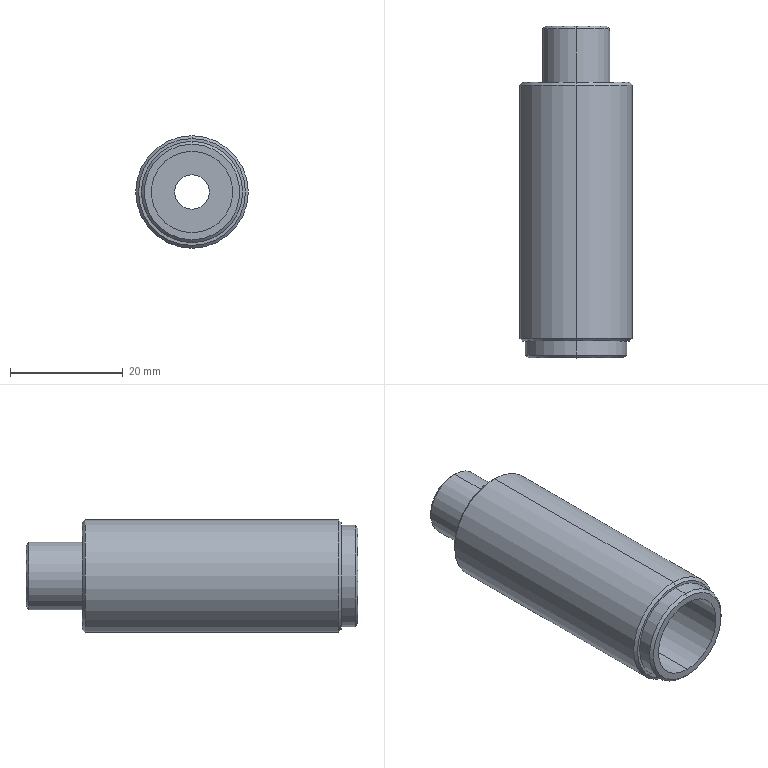Part | STEP file | 1 solid | 23 faces | box 20 x 59 x 20 mm | volume 11876 mm3 | cylinder 10 | cone 8 | plane 5 | commonest cylinder face diameters 6.1 x2 12 x2 14.5 x2 18 x2 20 x2
STEP:
#1=CARTESIAN_POINT('',(0.,0.,0.));
#2=DIRECTION('',(0.,0.,1.));
#3=DIRECTION('',(1.,0.,0.));
#4=AXIS2_PLACEMENT_3D('',#1,#2,#3);
#5=CARTESIAN_POINT('',(0.,10.,5.5));
#6=VERTEX_POINT('',#5);
#7=CARTESIAN_POINT('',(0.,10.,-5.5));
#8=VERTEX_POINT('',#7);
#9=CARTESIAN_POINT('',(0.,10.,0.));
#10=DIRECTION('',(0.,1.,0.));
#11=DIRECTION('',(0.,0.,1.));
#12=AXIS2_PLACEMENT_3D('',#9,#10,#11);
#13=CIRCLE('',#12,5.5);
#14=CARTESIAN_POINT('',(0.,10.,0.));
#15=DIRECTION('',(0.,-1.,0.));
#16=DIRECTION('',(0.,0.,-1.));
#17=AXIS2_PLACEMENT_3D('',#14,#15,#16);
#18=CONICAL_SURFACE('',#17,5.5,0.7854);
#19=CARTESIAN_POINT('',(3.142,0.));
#20=DIRECTION('',(-1.,0.));
#21=VECTOR('',#20,1.);
#22=LINE('',#19,#21);
#23=(GEOMETRIC_REPRESENTATION_CONTEXT(2)PARAMETRIC_REPRESENTATION_CONTEXT()REPRESENTATION_CONTEXT('',''));
#24=DEFINITIONAL_REPRESENTATION('',(#22),#23);
#25=PCURVE('',#18,#24);
#26=CARTESIAN_POINT('',(0.,10.,0.));
#27=DIRECTION('',(0.,1.,0.));
#28=DIRECTION('',(0.,0.,1.));
#29=AXIS2_PLACEMENT_3D('',#26,#27,#28);
#30=PLANE('',#29);
#31=CARTESIAN_POINT('',(0.,0.));
#32=DIRECTION('',(1.,0.));
#33=AXIS2_PLACEMENT_2D('',#31,#32);
#34=CIRCLE('',#33,5.5);
#35=(GEOMETRIC_REPRESENTATION_CONTEXT(2)PARAMETRIC_REPRESENTATION_CONTEXT()REPRESENTATION_CONTEXT('',''));
#36=DEFINITIONAL_REPRESENTATION('',(#34),#35);
#37=PCURVE('',#30,#36);
#38=SURFACE_CURVE('',#13,(#25,#37),.PCURVE_S1.);
#39=EDGE_CURVE('',#6,#8,#38,.T.);
#40=ORIENTED_EDGE('',*,*,#39,.F.);
#41=CARTESIAN_POINT('',(0.,9.5,6.));
#42=VERTEX_POINT('',#41);
#43=CARTESIAN_POINT('',(0.,10.,5.5));
#44=DIRECTION('',(0.,-0.7071,0.7071));
#45=VECTOR('',#44,1.);
#46=LINE('',#43,#45);
#47=CARTESIAN_POINT('',(3.142,0.));
#48=DIRECTION('',(0.,1.));
#49=VECTOR('',#48,1.);
#50=LINE('',#47,#49);
#51=(GEOMETRIC_REPRESENTATION_CONTEXT(2)PARAMETRIC_REPRESENTATION_CONTEXT()REPRESENTATION_CONTEXT('',''));
#52=DEFINITIONAL_REPRESENTATION('',(#50),#51);
#53=PCURVE('',#18,#52);
#54=CARTESIAN_POINT('',(0.,10.,0.));
#55=DIRECTION('',(0.,-1.,0.));
#56=DIRECTION('',(0.,0.,-1.));
#57=AXIS2_PLACEMENT_3D('',#54,#55,#56);
#58=CONICAL_SURFACE('',#57,5.5,0.7854);
#59=CARTESIAN_POINT('',(3.142,0.));
#60=DIRECTION('',(0.,1.));
#61=VECTOR('',#60,1.);
#62=LINE('',#59,#61);
#63=(GEOMETRIC_REPRESENTATION_CONTEXT(2)PARAMETRIC_REPRESENTATION_CONTEXT()REPRESENTATION_CONTEXT('',''));
#64=DEFINITIONAL_REPRESENTATION('',(#62),#63);
#65=PCURVE('',#58,#64);
#66=SURFACE_CURVE('',#46,(#53,#65),.PCURVE_S1.);
#67=EDGE_CURVE('',#6,#42,#66,.T.);
#68=ORIENTED_EDGE('',*,*,#67,.T.);
#69=CARTESIAN_POINT('',(0.,9.5,-6.));
#70=VERTEX_POINT('',#69);
#71=CARTESIAN_POINT('',(0.,9.5,0.));
#72=DIRECTION('',(0.,-1.,0.));
#73=DIRECTION('',(0.,0.,1.));
#74=AXIS2_PLACEMENT_3D('',#71,#72,#73);
#75=CIRCLE('',#74,6.);
#76=CARTESIAN_POINT('',(-3.142,0.5));
#77=DIRECTION('',(1.,0.));
#78=VECTOR('',#77,1.);
#79=LINE('',#76,#78);
#80=(GEOMETRIC_REPRESENTATION_CONTEXT(2)PARAMETRIC_REPRESENTATION_CONTEXT()REPRESENTATION_CONTEXT('',''));
#81=DEFINITIONAL_REPRESENTATION('',(#79),#80);
#82=PCURVE('',#18,#81);
#83=CARTESIAN_POINT('',(0.,10.,0.));
#84=DIRECTION('',(0.,-1.,0.));
#85=DIRECTION('',(0.,0.,-1.));
#86=AXIS2_PLACEMENT_3D('',#83,#84,#85);
#87=CYLINDRICAL_SURFACE('',#86,6.);
#88=CARTESIAN_POINT('',(-3.142,0.5));
#89=DIRECTION('',(1.,0.));
#90=VECTOR('',#89,1.);
#91=LINE('',#88,#90);
#92=(GEOMETRIC_REPRESENTATION_CONTEXT(2)PARAMETRIC_REPRESENTATION_CONTEXT()REPRESENTATION_CONTEXT('',''));
#93=DEFINITIONAL_REPRESENTATION('',(#91),#92);
#94=PCURVE('',#87,#93);
#95=SURFACE_CURVE('',#75,(#82,#94),.PCURVE_S1.);
#96=EDGE_CURVE('',#70,#42,#95,.T.);
#97=ORIENTED_EDGE('',*,*,#96,.F.);
#98=CARTESIAN_POINT('',(0.,10.,-5.5));
#99=DIRECTION('',(0.,-0.7071,-0.7071));
#100=VECTOR('',#99,1.);
#101=LINE('',#98,#100);
#102=CARTESIAN_POINT('',(0.,0.));
#103=DIRECTION('',(0.,1.));
#104=VECTOR('',#103,1.);
#105=LINE('',#102,#104);
#106=(GEOMETRIC_REPRESENTATION_CONTEXT(2)PARAMETRIC_REPRESENTATION_CONTEXT()REPRESENTATION_CONTEXT('',''));
#107=DEFINITIONAL_REPRESENTATION('',(#105),#106);
#108=PCURVE('',#18,#107);
#109=CARTESIAN_POINT('',(6.283,0.));
#110=DIRECTION('',(0.,1.));
#111=VECTOR('',#110,1.);
#112=LINE('',#109,#111);
#113=(GEOMETRIC_REPRESENTATION_CONTEXT(2)PARAMETRIC_REPRESENTATION_CONTEXT()REPRESENTATION_CONTEXT('',''));
#114=DEFINITIONAL_REPRESENTATION('',(#112),#113);
#115=PCURVE('',#58,#114);
#116=SURFACE_CURVE('',#101,(#108,#115),.PCURVE_S1.);
#117=EDGE_CURVE('',#8,#70,#116,.T.);
#118=ORIENTED_EDGE('',*,*,#117,.F.);
#119=EDGE_LOOP('',(#40,#68,#97,#118));
#120=FACE_BOUND('',#119,.T.);
#121=ADVANCED_FACE('',(#120),#18,.T.);
#122=CARTESIAN_POINT('',(0.,-49.,-8.5));
#123=VERTEX_POINT('',#122);
#124=CARTESIAN_POINT('',(0.,-49.,8.5));
#125=VERTEX_POINT('',#124);
#126=CARTESIAN_POINT('',(0.,-49.,0.));
#127=DIRECTION('',(0.,-1.,0.));
#128=DIRECTION('',(0.,0.,1.));
#129=AXIS2_PLACEMENT_3D('',#126,#127,#128);
#130=CIRCLE('',#129,8.5);
#131=CARTESIAN_POINT('',(0.,-49.,0.));
#132=DIRECTION('',(0.,1.,0.));
#133=DIRECTION('',(0.,0.,1.));
#134=AXIS2_PLACEMENT_3D('',#131,#132,#133);
#135=CONICAL_SURFACE('',#134,8.5,0.7854);
#136=CARTESIAN_POINT('',(6.283,0.));
#137=DIRECTION('',(-1.,0.));
#138=VECTOR('',#137,1.);
#139=LINE('',#136,#138);
#140=(GEOMETRIC_REPRESENTATION_CONTEXT(2)PARAMETRIC_REPRESENTATION_CONTEXT()REPRESENTATION_CONTEXT('',''));
#141=DEFINITIONAL_REPRESENTATION('',(#139),#140);
#142=PCURVE('',#135,#141);
#143=CARTESIAN_POINT('',(0.,-49.,0.));
#144=DIRECTION('',(0.,1.,0.));
#145=DIRECTION('',(0.,0.,1.));
#146=AXIS2_PLACEMENT_3D('',#143,#144,#145);
#147=PLANE('',#146);
#148=CARTESIAN_POINT('',(8.5,0.));
#149=CARTESIAN_POINT('',(8.5,-14.722));
#150=CARTESIAN_POINT('',(-4.25,-7.361));
#151=CARTESIAN_POINT('',(-17.,0.));
#152=CARTESIAN_POINT('',(-4.25,7.361));
#153=CARTESIAN_POINT('',(8.5,14.722));
#154=CARTESIAN_POINT('',(8.5,0.));
#155=(BOUNDED_CURVE()B_SPLINE_CURVE(2,(#148,#149,#150,#151,#152,#153,#154),.UNSPECIFIED.,.T.,.F.)B_SPLINE_CURVE_WITH_KNOTS((1,2,2,2,2,1),(-2.094,0.,2.094,4.189,6.283,8.378),.UNSPECIFIED.)CURVE()GEOMETRIC_REPRESENTATION_ITEM()RATIONAL_B_SPLINE_CURVE((1.,0.5,1.,0.5,1.,0.5,1.))REPRESENTATION_ITEM(''));
#156=(GEOMETRIC_REPRESENTATION_CONTEXT(2)PARAMETRIC_REPRESENTATION_CONTEXT()REPRESENTATION_CONTEXT('',''));
#157=DEFINITIONAL_REPRESENTATION('',(#155),#156);
#158=PCURVE('',#147,#157);
#159=SURFACE_CURVE('',#130,(#142,#158),.PCURVE_S1.);
#160=EDGE_CURVE('',#123,#125,#159,.T.);
#161=ORIENTED_EDGE('',*,*,#160,.F.);
#162=CARTESIAN_POINT('',(0.,-48.5,-9.));
#163=VERTEX_POINT('',#162);
#164=CARTESIAN_POINT('',(0.,-49.,-8.5));
#165=DIRECTION('',(0.,0.7071,-0.7071));
#166=VECTOR('',#165,1.);
#167=LINE('',#164,#166);
#168=CARTESIAN_POINT('',(3.142,0.));
#169=DIRECTION('',(0.,1.));
#170=VECTOR('',#169,1.);
#171=LINE('',#168,#170);
#172=(GEOMETRIC_REPRESENTATION_CONTEXT(2)PARAMETRIC_REPRESENTATION_CONTEXT()REPRESENTATION_CONTEXT('',''));
#173=DEFINITIONAL_REPRESENTATION('',(#171),#172);
#174=PCURVE('',#135,#173);
#175=CARTESIAN_POINT('',(0.,-49.,0.));
#176=DIRECTION('',(0.,1.,0.));
#177=DIRECTION('',(0.,0.,1.));
#178=AXIS2_PLACEMENT_3D('',#175,#176,#177);
#179=CONICAL_SURFACE('',#178,8.5,0.7854);
#180=CARTESIAN_POINT('',(3.142,0.));
#181=DIRECTION('',(0.,1.));
#182=VECTOR('',#181,1.);
#183=LINE('',#180,#182);
#184=(GEOMETRIC_REPRESENTATION_CONTEXT(2)PARAMETRIC_REPRESENTATION_CONTEXT()REPRESENTATION_CONTEXT('',''));
#185=DEFINITIONAL_REPRESENTATION('',(#183),#184);
#186=PCURVE('',#179,#185);
#187=SURFACE_CURVE('',#167,(#174,#186),.PCURVE_S1.);
#188=EDGE_CURVE('',#123,#163,#187,.T.);
#189=ORIENTED_EDGE('',*,*,#188,.T.);
#190=CARTESIAN_POINT('',(0.,-48.5,9.));
#191=VERTEX_POINT('',#190);
#192=CARTESIAN_POINT('',(0.,-48.5,0.));
#193=DIRECTION('',(0.,1.,0.));
#194=DIRECTION('',(0.,0.,1.));
#195=AXIS2_PLACEMENT_3D('',#192,#193,#194);
#196=CIRCLE('',#195,9.);
#197=CARTESIAN_POINT('',(0.,0.5));
#198=DIRECTION('',(1.,0.));
#199=VECTOR('',#198,1.);
#200=LINE('',#197,#199);
#201=(GEOMETRIC_REPRESENTATION_CONTEXT(2)PARAMETRIC_REPRESENTATION_CONTEXT()REPRESENTATION_CONTEXT('',''));
#202=DEFINITIONAL_REPRESENTATION('',(#200),#201);
#203=PCURVE('',#135,#202);
#204=CARTESIAN_POINT('',(0.,-46.,0.));
#205=DIRECTION('',(0.,-1.,0.));
#206=DIRECTION('',(0.,0.,-1.));
#207=AXIS2_PLACEMENT_3D('',#204,#205,#206);
#208=CYLINDRICAL_SURFACE('',#207,9.);
#209=CARTESIAN_POINT('',(3.142,2.5));
#210=DIRECTION('',(-1.,0.));
#211=VECTOR('',#210,1.);
#212=LINE('',#209,#211);
#213=(GEOMETRIC_REPRESENTATION_CONTEXT(2)PARAMETRIC_REPRESENTATION_CONTEXT()REPRESENTATION_CONTEXT('',''));
#214=DEFINITIONAL_REPRESENTATION('',(#212),#213);
#215=PCURVE('',#208,#214);
#216=SURFACE_CURVE('',#196,(#203,#215),.PCURVE_S1.);
#217=EDGE_CURVE('',#191,#163,#216,.T.);
#218=ORIENTED_EDGE('',*,*,#217,.F.);
#219=CARTESIAN_POINT('',(0.,-49.,8.5));
#220=DIRECTION('',(0.,0.7071,0.7071));
#221=VECTOR('',#220,1.);
#222=LINE('',#219,#221);
#223=CARTESIAN_POINT('',(0.,0.));
#224=DIRECTION('',(0.,1.));
#225=VECTOR('',#224,1.);
#226=LINE('',#223,#225);
#227=(GEOMETRIC_REPRESENTATION_CONTEXT(2)PARAMETRIC_REPRESENTATION_CONTEXT()REPRESENTATION_CONTEXT('',''));
#228=DEFINITIONAL_REPRESENTATION('',(#226),#227);
#229=PCURVE('',#135,#228);
#230=CARTESIAN_POINT('',(6.283,0.));
#231=DIRECTION('',(0.,1.));
#232=VECTOR('',#231,1.);
#233=LINE('',#230,#232);
#234=(GEOMETRIC_REPRESENTATION_CONTEXT(2)PARAMETRIC_REPRESENTATION_CONTEXT()REPRESENTATION_CONTEXT('',''));
#235=DEFINITIONAL_REPRESENTATION('',(#233),#234);
#236=PCURVE('',#179,#235);
#237=SURFACE_CURVE('',#222,(#229,#236),.PCURVE_S1.);
#238=EDGE_CURVE('',#125,#191,#237,.T.);
#239=ORIENTED_EDGE('',*,*,#238,.F.);
#240=EDGE_LOOP('',(#161,#189,#218,#239));
#241=FACE_BOUND('',#240,.T.);
#242=ADVANCED_FACE('',(#241),#135,.T.);
#243=CARTESIAN_POINT('',(0.,0.,9.5));
#244=VERTEX_POINT('',#243);
#245=CARTESIAN_POINT('',(0.,0.,-9.5));
#246=VERTEX_POINT('',#245);
#247=CARTESIAN_POINT('',(0.,0.,0.));
#248=DIRECTION('',(0.,1.,0.));
#249=DIRECTION('',(0.,0.,1.));
#250=AXIS2_PLACEMENT_3D('',#247,#248,#249);
#251=CIRCLE('',#250,9.5);
#252=CARTESIAN_POINT('',(0.,0.,0.));
#253=DIRECTION('',(0.,-1.,0.));
#254=DIRECTION('',(0.,0.,-1.));
#255=AXIS2_PLACEMENT_3D('',#252,#253,#254);
#256=CONICAL_SURFACE('',#255,9.5,0.7854);
#257=CARTESIAN_POINT('',(3.142,0.));
#258=DIRECTION('',(-1.,0.));
#259=VECTOR('',#258,1.);
#260=LINE('',#257,#259);
#261=(GEOMETRIC_REPRESENTATION_CONTEXT(2)PARAMETRIC_REPRESENTATION_CONTEXT()REPRESENTATION_CONTEXT('',''));
#262=DEFINITIONAL_REPRESENTATION('',(#260),#261);
#263=PCURVE('',#256,#262);
#264=CARTESIAN_POINT('',(0.,0.,0.));
#265=DIRECTION('',(0.,1.,0.));
#266=DIRECTION('',(0.,0.,1.));
#267=AXIS2_PLACEMENT_3D('',#264,#265,#266);
#268=PLANE('',#267);
#269=CARTESIAN_POINT('',(0.,0.));
#270=DIRECTION('',(1.,0.));
#271=AXIS2_PLACEMENT_2D('',#269,#270);
#272=CIRCLE('',#271,9.5);
#273=(GEOMETRIC_REPRESENTATION_CONTEXT(2)PARAMETRIC_REPRESENTATION_CONTEXT()REPRESENTATION_CONTEXT('',''));
#274=DEFINITIONAL_REPRESENTATION('',(#272),#273);
#275=PCURVE('',#268,#274);
#276=SURFACE_CURVE('',#251,(#263,#275),.PCURVE_S1.);
#277=EDGE_CURVE('',#244,#246,#276,.T.);
#278=ORIENTED_EDGE('',*,*,#277,.F.);
#279=CARTESIAN_POINT('',(0.,-0.5,10.));
#280=VERTEX_POINT('',#279);
#281=CARTESIAN_POINT('',(0.,0.,9.5));
#282=DIRECTION('',(0.,-0.7071,0.7071));
#283=VECTOR('',#282,1.);
#284=LINE('',#281,#283);
#285=CARTESIAN_POINT('',(3.142,0.));
#286=DIRECTION('',(0.,1.));
#287=VECTOR('',#286,1.);
#288=LINE('',#285,#287);
#289=(GEOMETRIC_REPRESENTATION_CONTEXT(2)PARAMETRIC_REPRESENTATION_CONTEXT()REPRESENTATION_CONTEXT('',''));
#290=DEFINITIONAL_REPRESENTATION('',(#288),#289);
#291=PCURVE('',#256,#290);
#292=CARTESIAN_POINT('',(0.,0.,0.));
#293=DIRECTION('',(0.,-1.,0.));
#294=DIRECTION('',(0.,0.,-1.));
#295=AXIS2_PLACEMENT_3D('',#292,#293,#294);
#296=CONICAL_SURFACE('',#295,9.5,0.7854);
#297=CARTESIAN_POINT('',(3.142,0.));
#298=DIRECTION('',(0.,1.));
#299=VECTOR('',#298,1.);
#300=LINE('',#297,#299);
#301=(GEOMETRIC_REPRESENTATION_CONTEXT(2)PARAMETRIC_REPRESENTATION_CONTEXT()REPRESENTATION_CONTEXT('',''));
#302=DEFINITIONAL_REPRESENTATION('',(#300),#301);
#303=PCURVE('',#296,#302);
#304=SURFACE_CURVE('',#284,(#291,#303),.PCURVE_S1.);
#305=EDGE_CURVE('',#244,#280,#304,.T.);
#306=ORIENTED_EDGE('',*,*,#305,.T.);
#307=CARTESIAN_POINT('',(0.,-0.5,-10.));
#308=VERTEX_POINT('',#307);
#309=CARTESIAN_POINT('',(0.,-0.5,0.));
#310=DIRECTION('',(0.,-1.,0.));
#311=DIRECTION('',(0.,0.,1.));
#312=AXIS2_PLACEMENT_3D('',#309,#310,#311);
#313=CIRCLE('',#312,10.);
#314=CARTESIAN_POINT('',(-3.142,0.5));
#315=DIRECTION('',(1.,0.));
#316=VECTOR('',#315,1.);
#317=LINE('',#314,#316);
#318=(GEOMETRIC_REPRESENTATION_CONTEXT(2)PARAMETRIC_REPRESENTATION_CONTEXT()REPRESENTATION_CONTEXT('',''));
#319=DEFINITIONAL_REPRESENTATION('',(#317),#318);
#320=PCURVE('',#256,#319);
#321=CARTESIAN_POINT('',(0.,-49.,0.));
#322=DIRECTION('',(0.,1.,0.));
#323=DIRECTION('',(0.,0.,1.));
#324=AXIS2_PLACEMENT_3D('',#321,#322,#323);
#325=CYLINDRICAL_SURFACE('',#324,10.);
#326=CARTESIAN_POINT('',(6.283,48.5));
#327=DIRECTION('',(-1.,0.));
#328=VECTOR('',#327,1.);
#329=LINE('',#326,#328);
#330=(GEOMETRIC_REPRESENTATION_CONTEXT(2)PARAMETRIC_REPRESENTATION_CONTEXT()REPRESENTATION_CONTEXT('',''));
#331=DEFINITIONAL_REPRESENTATION('',(#329),#330);
#332=PCURVE('',#325,#331);
#333=SURFACE_CURVE('',#313,(#320,#332),.PCURVE_S1.);
#334=EDGE_CURVE('',#308,#280,#333,.T.);
#335=ORIENTED_EDGE('',*,*,#334,.F.);
#336=CARTESIAN_POINT('',(0.,0.,-9.5));
#337=DIRECTION('',(0.,-0.7071,-0.7071));
#338=VECTOR('',#337,1.);
#339=LINE('',#336,#338);
#340=CARTESIAN_POINT('',(0.,0.));
#341=DIRECTION('',(0.,1.));
#342=VECTOR('',#341,1.);
#343=LINE('',#340,#342);
#344=(GEOMETRIC_REPRESENTATION_CONTEXT(2)PARAMETRIC_REPRESENTATION_CONTEXT()REPRESENTATION_CONTEXT('',''));
#345=DEFINITIONAL_REPRESENTATION('',(#343),#344);
#346=PCURVE('',#256,#345);
#347=CARTESIAN_POINT('',(6.283,0.));
#348=DIRECTION('',(0.,1.));
#349=VECTOR('',#348,1.);
#350=LINE('',#347,#349);
#351=(GEOMETRIC_REPRESENTATION_CONTEXT(2)PARAMETRIC_REPRESENTATION_CONTEXT()REPRESENTATION_CONTEXT('',''));
#352=DEFINITIONAL_REPRESENTATION('',(#350),#351);
#353=PCURVE('',#296,#352);
#354=SURFACE_CURVE('',#339,(#346,#353),.PCURVE_S1.);
#355=EDGE_CURVE('',#246,#308,#354,.T.);
#356=ORIENTED_EDGE('',*,*,#355,.F.);
#357=EDGE_LOOP('',(#278,#306,#335,#356));
#358=FACE_BOUND('',#357,.T.);
#359=ADVANCED_FACE('',(#358),#256,.T.);
#360=CARTESIAN_POINT('',(0.,-46.,-9.5));
#361=VERTEX_POINT('',#360);
#362=CARTESIAN_POINT('',(0.,-46.,9.5));
#363=VERTEX_POINT('',#362);
#364=CARTESIAN_POINT('',(0.,-46.,0.));
#365=DIRECTION('',(0.,-1.,0.));
#366=DIRECTION('',(0.,0.,-1.));
#367=AXIS2_PLACEMENT_3D('',#364,#365,#366);
#368=CIRCLE('',#367,9.5);
#369=CARTESIAN_POINT('',(0.,-46.,0.));
#370=DIRECTION('',(0.,1.,0.));
#371=DIRECTION('',(0.,0.,1.));
#372=AXIS2_PLACEMENT_3D('',#369,#370,#371);
#373=CONICAL_SURFACE('',#372,9.5,0.7854);
#374=CARTESIAN_POINT('',(3.142,0.));
#375=DIRECTION('',(-1.,0.));
#376=VECTOR('',#375,1.);
#377=LINE('',#374,#376);
#378=(GEOMETRIC_REPRESENTATION_CONTEXT(2)PARAMETRIC_REPRESENTATION_CONTEXT()REPRESENTATION_CONTEXT('',''));
#379=DEFINITIONAL_REPRESENTATION('',(#377),#378);
#380=PCURVE('',#373,#379);
#381=CARTESIAN_POINT('',(0.,-46.,0.));
#382=DIRECTION('',(0.,-1.,0.));
#383=DIRECTION('',(0.,0.,-1.));
#384=AXIS2_PLACEMENT_3D('',#381,#382,#383);
#385=PLANE('',#384);
#386=CARTESIAN_POINT('',(0.,0.));
#387=DIRECTION('',(1.,0.));
#388=AXIS2_PLACEMENT_2D('',#386,#387);
#389=CIRCLE('',#388,9.5);
#390=(GEOMETRIC_REPRESENTATION_CONTEXT(2)PARAMETRIC_REPRESENTATION_CONTEXT()REPRESENTATION_CONTEXT('',''));
#391=DEFINITIONAL_REPRESENTATION('',(#389),#390);
#392=PCURVE('',#385,#391);
#393=SURFACE_CURVE('',#368,(#380,#392),.PCURVE_S1.);
#394=EDGE_CURVE('',#361,#363,#393,.T.);
#395=ORIENTED_EDGE('',*,*,#394,.F.);
#396=CARTESIAN_POINT('',(0.,-45.5,-10.));
#397=VERTEX_POINT('',#396);
#398=CARTESIAN_POINT('',(0.,-46.,-9.5));
#399=DIRECTION('',(0.,0.7071,-0.7071));
#400=VECTOR('',#399,1.);
#401=LINE('',#398,#400);
#402=CARTESIAN_POINT('',(3.142,0.));
#403=DIRECTION('',(0.,1.));
#404=VECTOR('',#403,1.);
#405=LINE('',#402,#404);
#406=(GEOMETRIC_REPRESENTATION_CONTEXT(2)PARAMETRIC_REPRESENTATION_CONTEXT()REPRESENTATION_CONTEXT('',''));
#407=DEFINITIONAL_REPRESENTATION('',(#405),#406);
#408=PCURVE('',#373,#407);
#409=CARTESIAN_POINT('',(0.,-46.,0.));
#410=DIRECTION('',(0.,1.,0.));
#411=DIRECTION('',(0.,0.,1.));
#412=AXIS2_PLACEMENT_3D('',#409,#410,#411);
#413=CONICAL_SURFACE('',#412,9.5,0.7854);
#414=CARTESIAN_POINT('',(3.142,0.));
#415=DIRECTION('',(0.,1.));
#416=VECTOR('',#415,1.);
#417=LINE('',#414,#416);
#418=(GEOMETRIC_REPRESENTATION_CONTEXT(2)PARAMETRIC_REPRESENTATION_CONTEXT()REPRESENTATION_CONTEXT('',''));
#419=DEFINITIONAL_REPRESENTATION('',(#417),#418);
#420=PCURVE('',#413,#419);
#421=SURFACE_CURVE('',#401,(#408,#420),.PCURVE_S1.);
#422=EDGE_CURVE('',#361,#397,#421,.T.);
#423=ORIENTED_EDGE('',*,*,#422,.T.);
#424=CARTESIAN_POINT('',(0.,-45.5,10.));
#425=VERTEX_POINT('',#424);
#426=CARTESIAN_POINT('',(0.,-45.5,0.));
#427=DIRECTION('',(0.,1.,0.));
#428=DIRECTION('',(0.,0.,-1.));
#429=AXIS2_PLACEMENT_3D('',#426,#427,#428);
#430=CIRCLE('',#429,10.);
#431=CARTESIAN_POINT('',(-3.142,0.5));
#432=DIRECTION('',(1.,0.));
#433=VECTOR('',#432,1.);
#434=LINE('',#431,#433);
#435=(GEOMETRIC_REPRESENTATION_CONTEXT(2)PARAMETRIC_REPRESENTATION_CONTEXT()REPRESENTATION_CONTEXT('',''));
#436=DEFINITIONAL_REPRESENTATION('',(#434),#435);
#437=PCURVE('',#373,#436);
#438=CARTESIAN_POINT('',(-3.142,3.5));
#439=DIRECTION('',(1.,0.));
#440=VECTOR('',#439,1.);
#441=LINE('',#438,#440);
#442=(GEOMETRIC_REPRESENTATION_CONTEXT(2)PARAMETRIC_REPRESENTATION_CONTEXT()REPRESENTATION_CONTEXT('',''));
#443=DEFINITIONAL_REPRESENTATION('',(#441),#442);
#444=PCURVE('',#325,#443);
#445=SURFACE_CURVE('',#430,(#437,#444),.PCURVE_S1.);
#446=EDGE_CURVE('',#425,#397,#445,.T.);
#447=ORIENTED_EDGE('',*,*,#446,.F.);
#448=CARTESIAN_POINT('',(0.,-46.,9.5));
#449=DIRECTION('',(0.,0.7071,0.7071));
#450=VECTOR('',#449,1.);
#451=LINE('',#448,#450);
#452=CARTESIAN_POINT('',(0.,0.));
#453=DIRECTION('',(0.,1.));
#454=VECTOR('',#453,1.);
#455=LINE('',#452,#454);
#456=(GEOMETRIC_REPRESENTATION_CONTEXT(2)PARAMETRIC_REPRESENTATION_CONTEXT()REPRESENTATION_CONTEXT('',''));
#457=DEFINITIONAL_REPRESENTATION('',(#455),#456);
#458=PCURVE('',#373,#457);
#459=CARTESIAN_POINT('',(6.283,0.));
#460=DIRECTION('',(0.,1.));
#461=VECTOR('',#460,1.);
#462=LINE('',#459,#461);
#463=(GEOMETRIC_REPRESENTATION_CONTEXT(2)PARAMETRIC_REPRESENTATION_CONTEXT()REPRESENTATION_CONTEXT('',''));
#464=DEFINITIONAL_REPRESENTATION('',(#462),#463);
#465=PCURVE('',#413,#464);
#466=SURFACE_CURVE('',#451,(#458,#465),.PCURVE_S1.);
#467=EDGE_CURVE('',#363,#425,#466,.T.);
#468=ORIENTED_EDGE('',*,*,#467,.F.);
#469=EDGE_LOOP('',(#395,#423,#447,#468));
#470=FACE_BOUND('',#469,.T.);
#471=ADVANCED_FACE('',(#470),#373,.T.);
#472=CARTESIAN_POINT('',(0.,-46.,-9.));
#473=VERTEX_POINT('',#472);
#474=CARTESIAN_POINT('',(0.,-46.,9.));
#475=VERTEX_POINT('',#474);
#476=CARTESIAN_POINT('',(0.,-46.,0.));
#477=DIRECTION('',(0.,-1.,0.));
#478=DIRECTION('',(0.,0.,-1.));
#479=AXIS2_PLACEMENT_3D('',#476,#477,#478);
#480=CIRCLE('',#479,9.);
#481=CARTESIAN_POINT('',(0.,0.));
#482=DIRECTION('',(1.,0.));
#483=VECTOR('',#482,1.);
#484=LINE('',#481,#483);
#485=(GEOMETRIC_REPRESENTATION_CONTEXT(2)PARAMETRIC_REPRESENTATION_CONTEXT()REPRESENTATION_CONTEXT('',''));
#486=DEFINITIONAL_REPRESENTATION('',(#484),#485);
#487=PCURVE('',#208,#486);
#488=CARTESIAN_POINT('',(0.,0.));
#489=DIRECTION('',(1.,0.));
#490=AXIS2_PLACEMENT_2D('',#488,#489);
#491=CIRCLE('',#490,9.);
#492=(GEOMETRIC_REPRESENTATION_CONTEXT(2)PARAMETRIC_REPRESENTATION_CONTEXT()REPRESENTATION_CONTEXT('',''));
#493=DEFINITIONAL_REPRESENTATION('',(#491),#492);
#494=PCURVE('',#385,#493);
#495=SURFACE_CURVE('',#480,(#487,#494),.PCURVE_S1.);
#496=EDGE_CURVE('',#473,#475,#495,.T.);
#497=ORIENTED_EDGE('',*,*,#496,.T.);
#498=CARTESIAN_POINT('',(0.,-46.,9.));
#499=DIRECTION('',(0.,-1.,0.));
#500=VECTOR('',#499,1.);
#501=LINE('',#498,#500);
#502=CARTESIAN_POINT('',(3.142,0.));
#503=DIRECTION('',(0.,1.));
#504=VECTOR('',#503,1.);
#505=LINE('',#502,#504);
#506=(GEOMETRIC_REPRESENTATION_CONTEXT(2)PARAMETRIC_REPRESENTATION_CONTEXT()REPRESENTATION_CONTEXT('',''));
#507=DEFINITIONAL_REPRESENTATION('',(#505),#506);
#508=PCURVE('',#208,#507);
#509=CARTESIAN_POINT('',(0.,-46.,0.));
#510=DIRECTION('',(0.,-1.,0.));
#511=DIRECTION('',(0.,0.,-1.));
#512=AXIS2_PLACEMENT_3D('',#509,#510,#511);
#513=CYLINDRICAL_SURFACE('',#512,9.);
#514=CARTESIAN_POINT('',(3.142,0.));
#515=DIRECTION('',(0.,1.));
#516=VECTOR('',#515,1.);
#517=LINE('',#514,#516);
#518=(GEOMETRIC_REPRESENTATION_CONTEXT(2)PARAMETRIC_REPRESENTATION_CONTEXT()REPRESENTATION_CONTEXT('',''));
#519=DEFINITIONAL_REPRESENTATION('',(#517),#518);
#520=PCURVE('',#513,#519);
#521=SURFACE_CURVE('',#501,(#508,#520),.PCURVE_S1.);
#522=EDGE_CURVE('',#475,#191,#521,.T.);
#523=ORIENTED_EDGE('',*,*,#522,.T.);
#524=ORIENTED_EDGE('',*,*,#217,.T.);
#525=CARTESIAN_POINT('',(0.,-46.,-9.));
#526=DIRECTION('',(0.,-1.,0.));
#527=VECTOR('',#526,1.);
#528=LINE('',#525,#527);
#529=CARTESIAN_POINT('',(0.,0.));
#530=DIRECTION('',(0.,1.));
#531=VECTOR('',#530,1.);
#532=LINE('',#529,#531);
#533=(GEOMETRIC_REPRESENTATION_CONTEXT(2)PARAMETRIC_REPRESENTATION_CONTEXT()REPRESENTATION_CONTEXT('',''));
#534=DEFINITIONAL_REPRESENTATION('',(#532),#533);
#535=PCURVE('',#208,#534);
#536=CARTESIAN_POINT('',(6.283,0.));
#537=DIRECTION('',(0.,1.));
#538=VECTOR('',#537,1.);
#539=LINE('',#536,#538);
#540=(GEOMETRIC_REPRESENTATION_CONTEXT(2)PARAMETRIC_REPRESENTATION_CONTEXT()REPRESENTATION_CONTEXT('',''));
#541=DEFINITIONAL_REPRESENTATION('',(#539),#540);
#542=PCURVE('',#513,#541);
#543=SURFACE_CURVE('',#528,(#535,#542),.PCURVE_S1.);
#544=EDGE_CURVE('',#473,#163,#543,.T.);
#545=ORIENTED_EDGE('',*,*,#544,.F.);
#546=EDGE_LOOP('',(#497,#523,#524,#545));
#547=FACE_BOUND('',#546,.T.);
#548=ADVANCED_FACE('',(#547),#208,.T.);
#549=CARTESIAN_POINT('',(0.,-29.,-7.25));
#550=VERTEX_POINT('',#549);
#551=CARTESIAN_POINT('',(0.,-49.,-7.25));
#552=VERTEX_POINT('',#551);
#553=CARTESIAN_POINT('',(0.,-29.,-7.25));
#554=DIRECTION('',(0.,-1.,0.));
#555=VECTOR('',#554,1.);
#556=LINE('',#553,#555);
#557=CARTESIAN_POINT('',(0.,-29.,0.));
#558=DIRECTION('',(0.,-1.,0.));
#559=DIRECTION('',(0.,0.,-1.));
#560=AXIS2_PLACEMENT_3D('',#557,#558,#559);
#561=CYLINDRICAL_SURFACE('',#560,7.25);
#562=CARTESIAN_POINT('',(6.283,0.));
#563=DIRECTION('',(0.,1.));
#564=VECTOR('',#563,1.);
#565=LINE('',#562,#564);
#566=(GEOMETRIC_REPRESENTATION_CONTEXT(2)PARAMETRIC_REPRESENTATION_CONTEXT()REPRESENTATION_CONTEXT('',''));
#567=DEFINITIONAL_REPRESENTATION('',(#565),#566);
#568=PCURVE('',#561,#567);
#569=CARTESIAN_POINT('',(0.,-29.,0.));
#570=DIRECTION('',(0.,-1.,0.));
#571=DIRECTION('',(0.,0.,-1.));
#572=AXIS2_PLACEMENT_3D('',#569,#570,#571);
#573=CYLINDRICAL_SURFACE('',#572,7.25);
#574=CARTESIAN_POINT('',(0.,0.));
#575=DIRECTION('',(0.,1.));
#576=VECTOR('',#575,1.);
#577=LINE('',#574,#576);
#578=(GEOMETRIC_REPRESENTATION_CONTEXT(2)PARAMETRIC_REPRESENTATION_CONTEXT()REPRESENTATION_CONTEXT('',''));
#579=DEFINITIONAL_REPRESENTATION('',(#577),#578);
#580=PCURVE('',#573,#579);
#581=SURFACE_CURVE('',#556,(#568,#580),.PCURVE_S1.);
#582=EDGE_CURVE('',#550,#552,#581,.T.);
#583=ORIENTED_EDGE('',*,*,#582,.T.);
#584=CARTESIAN_POINT('',(0.,-49.,7.25));
#585=VERTEX_POINT('',#584);
#586=CARTESIAN_POINT('',(0.,-49.,0.));
#587=DIRECTION('',(0.,-1.,0.));
#588=DIRECTION('',(0.,0.,-1.));
#589=AXIS2_PLACEMENT_3D('',#586,#587,#588);
#590=CIRCLE('',#589,7.25);
#591=CARTESIAN_POINT('',(0.,20.));
#592=DIRECTION('',(1.,0.));
#593=VECTOR('',#592,1.);
#594=LINE('',#591,#593);
#595=(GEOMETRIC_REPRESENTATION_CONTEXT(2)PARAMETRIC_REPRESENTATION_CONTEXT()REPRESENTATION_CONTEXT('',''));
#596=DEFINITIONAL_REPRESENTATION('',(#594),#595);
#597=PCURVE('',#561,#596);
#598=CARTESIAN_POINT('',(-7.25,0.));
#599=CARTESIAN_POINT('',(-7.25,12.557));
#600=CARTESIAN_POINT('',(3.625,6.279));
#601=CARTESIAN_POINT('',(14.5,0.));
#602=CARTESIAN_POINT('',(3.625,-6.279));
#603=CARTESIAN_POINT('',(-7.25,-12.557));
#604=CARTESIAN_POINT('',(-7.25,0.));
#605=(BOUNDED_CURVE()B_SPLINE_CURVE(2,(#598,#599,#600,#601,#602,#603,#604),.UNSPECIFIED.,.T.,.F.)B_SPLINE_CURVE_WITH_KNOTS((1,2,2,2,2,1),(-2.094,0.,2.094,4.189,6.283,8.378),.UNSPECIFIED.)CURVE()GEOMETRIC_REPRESENTATION_ITEM()RATIONAL_B_SPLINE_CURVE((1.,0.5,1.,0.5,1.,0.5,1.))REPRESENTATION_ITEM(''));
#606=(GEOMETRIC_REPRESENTATION_CONTEXT(2)PARAMETRIC_REPRESENTATION_CONTEXT()REPRESENTATION_CONTEXT('',''));
#607=DEFINITIONAL_REPRESENTATION('',(#605),#606);
#608=PCURVE('',#147,#607);
#609=SURFACE_CURVE('',#590,(#597,#608),.PCURVE_S1.);
#610=EDGE_CURVE('',#585,#552,#609,.T.);
#611=ORIENTED_EDGE('',*,*,#610,.F.);
#612=CARTESIAN_POINT('',(0.,-29.,7.25));
#613=VERTEX_POINT('',#612);
#614=CARTESIAN_POINT('',(0.,-29.,7.25));
#615=DIRECTION('',(0.,-1.,0.));
#616=VECTOR('',#615,1.);
#617=LINE('',#614,#616);
#618=CARTESIAN_POINT('',(3.142,0.));
#619=DIRECTION('',(0.,1.));
#620=VECTOR('',#619,1.);
#621=LINE('',#618,#620);
#622=(GEOMETRIC_REPRESENTATION_CONTEXT(2)PARAMETRIC_REPRESENTATION_CONTEXT()REPRESENTATION_CONTEXT('',''));
#623=DEFINITIONAL_REPRESENTATION('',(#621),#622);
#624=PCURVE('',#561,#623);
#625=CARTESIAN_POINT('',(3.142,0.));
#626=DIRECTION('',(0.,1.));
#627=VECTOR('',#626,1.);
#628=LINE('',#625,#627);
#629=(GEOMETRIC_REPRESENTATION_CONTEXT(2)PARAMETRIC_REPRESENTATION_CONTEXT()REPRESENTATION_CONTEXT('',''));
#630=DEFINITIONAL_REPRESENTATION('',(#628),#629);
#631=PCURVE('',#573,#630);
#632=SURFACE_CURVE('',#617,(#624,#631),.PCURVE_S1.);
#633=EDGE_CURVE('',#613,#585,#632,.T.);
#634=ORIENTED_EDGE('',*,*,#633,.F.);
#635=CARTESIAN_POINT('',(0.,-29.,0.));
#636=DIRECTION('',(0.,-1.,0.));
#637=DIRECTION('',(0.,0.,-1.));
#638=AXIS2_PLACEMENT_3D('',#635,#636,#637);
#639=CIRCLE('',#638,7.25);
#640=CARTESIAN_POINT('',(0.,0.));
#641=DIRECTION('',(1.,0.));
#642=VECTOR('',#641,1.);
#643=LINE('',#640,#642);
#644=(GEOMETRIC_REPRESENTATION_CONTEXT(2)PARAMETRIC_REPRESENTATION_CONTEXT()REPRESENTATION_CONTEXT('',''));
#645=DEFINITIONAL_REPRESENTATION('',(#643),#644);
#646=PCURVE('',#561,#645);
#647=CARTESIAN_POINT('',(0.,-29.,0.));
#648=DIRECTION('',(0.,-1.,0.));
#649=DIRECTION('',(0.,0.,-1.));
#650=AXIS2_PLACEMENT_3D('',#647,#648,#649);
#651=PLANE('',#650);
#652=CARTESIAN_POINT('',(0.,0.));
#653=DIRECTION('',(1.,0.));
#654=AXIS2_PLACEMENT_2D('',#652,#653);
#655=CIRCLE('',#654,7.25);
#656=(GEOMETRIC_REPRESENTATION_CONTEXT(2)PARAMETRIC_REPRESENTATION_CONTEXT()REPRESENTATION_CONTEXT('',''));
#657=DEFINITIONAL_REPRESENTATION('',(#655),#656);
#658=PCURVE('',#651,#657);
#659=SURFACE_CURVE('',#639,(#646,#658),.PCURVE_S1.);
#660=EDGE_CURVE('',#613,#550,#659,.T.);
#661=ORIENTED_EDGE('',*,*,#660,.T.);
#662=EDGE_LOOP('',(#583,#611,#634,#661));
#663=FACE_BOUND('',#662,.F.);
#664=ADVANCED_FACE('',(#663),#561,.F.);
#665=ORIENTED_EDGE('',*,*,#96,.T.);
#666=CARTESIAN_POINT('',(0.,0.,6.));
#667=VERTEX_POINT('',#666);
#668=CARTESIAN_POINT('',(0.,10.,6.));
#669=DIRECTION('',(0.,-1.,0.));
#670=VECTOR('',#669,1.);
#671=LINE('',#668,#670);
#672=CARTESIAN_POINT('',(3.142,0.));
#673=DIRECTION('',(0.,1.));
#674=VECTOR('',#673,1.);
#675=LINE('',#672,#674);
#676=(GEOMETRIC_REPRESENTATION_CONTEXT(2)PARAMETRIC_REPRESENTATION_CONTEXT()REPRESENTATION_CONTEXT('',''));
#677=DEFINITIONAL_REPRESENTATION('',(#675),#676);
#678=PCURVE('',#87,#677);
#679=CARTESIAN_POINT('',(0.,10.,0.));
#680=DIRECTION('',(0.,-1.,0.));
#681=DIRECTION('',(0.,0.,-1.));
#682=AXIS2_PLACEMENT_3D('',#679,#680,#681);
#683=CYLINDRICAL_SURFACE('',#682,6.);
#684=CARTESIAN_POINT('',(3.142,0.));
#685=DIRECTION('',(0.,1.));
#686=VECTOR('',#685,1.);
#687=LINE('',#684,#686);
#688=(GEOMETRIC_REPRESENTATION_CONTEXT(2)PARAMETRIC_REPRESENTATION_CONTEXT()REPRESENTATION_CONTEXT('',''));
#689=DEFINITIONAL_REPRESENTATION('',(#687),#688);
#690=PCURVE('',#683,#689);
#691=SURFACE_CURVE('',#671,(#678,#690),.PCURVE_S1.);
#692=EDGE_CURVE('',#42,#667,#691,.T.);
#693=ORIENTED_EDGE('',*,*,#692,.T.);
#694=CARTESIAN_POINT('',(0.,0.,-6.));
#695=VERTEX_POINT('',#694);
#696=CARTESIAN_POINT('',(0.,0.,0.));
#697=DIRECTION('',(0.,1.,0.));
#698=DIRECTION('',(0.,0.,1.));
#699=AXIS2_PLACEMENT_3D('',#696,#697,#698);
#700=CIRCLE('',#699,6.);
#701=CARTESIAN_POINT('',(3.142,10.));
#702=DIRECTION('',(-1.,0.));
#703=VECTOR('',#702,1.);
#704=LINE('',#701,#703);
#705=(GEOMETRIC_REPRESENTATION_CONTEXT(2)PARAMETRIC_REPRESENTATION_CONTEXT()REPRESENTATION_CONTEXT('',''));
#706=DEFINITIONAL_REPRESENTATION('',(#704),#705);
#707=PCURVE('',#87,#706);
#708=CARTESIAN_POINT('',(0.,0.));
#709=DIRECTION('',(1.,0.));
#710=AXIS2_PLACEMENT_2D('',#708,#709);
#711=CIRCLE('',#710,6.);
#712=(GEOMETRIC_REPRESENTATION_CONTEXT(2)PARAMETRIC_REPRESENTATION_CONTEXT()REPRESENTATION_CONTEXT('',''));
#713=DEFINITIONAL_REPRESENTATION('',(#711),#712);
#714=PCURVE('',#268,#713);
#715=SURFACE_CURVE('',#700,(#707,#714),.PCURVE_S1.);
#716=EDGE_CURVE('',#667,#695,#715,.T.);
#717=ORIENTED_EDGE('',*,*,#716,.T.);
#718=CARTESIAN_POINT('',(0.,10.,-6.));
#719=DIRECTION('',(0.,-1.,0.));
#720=VECTOR('',#719,1.);
#721=LINE('',#718,#720);
#722=CARTESIAN_POINT('',(0.,0.));
#723=DIRECTION('',(0.,1.));
#724=VECTOR('',#723,1.);
#725=LINE('',#722,#724);
#726=(GEOMETRIC_REPRESENTATION_CONTEXT(2)PARAMETRIC_REPRESENTATION_CONTEXT()REPRESENTATION_CONTEXT('',''));
#727=DEFINITIONAL_REPRESENTATION('',(#725),#726);
#728=PCURVE('',#87,#727);
#729=CARTESIAN_POINT('',(6.283,0.));
#730=DIRECTION('',(0.,1.));
#731=VECTOR('',#730,1.);
#732=LINE('',#729,#731);
#733=(GEOMETRIC_REPRESENTATION_CONTEXT(2)PARAMETRIC_REPRESENTATION_CONTEXT()REPRESENTATION_CONTEXT('',''));
#734=DEFINITIONAL_REPRESENTATION('',(#732),#733);
#735=PCURVE('',#683,#734);
#736=SURFACE_CURVE('',#721,(#728,#735),.PCURVE_S1.);
#737=EDGE_CURVE('',#70,#695,#736,.T.);
#738=ORIENTED_EDGE('',*,*,#737,.F.);
#739=EDGE_LOOP('',(#665,#693,#717,#738));
#740=FACE_BOUND('',#739,.T.);
#741=ADVANCED_FACE('',(#740),#87,.T.);
#742=CARTESIAN_POINT('',(0.,-29.,3.05));
#743=VERTEX_POINT('',#742);
#744=CARTESIAN_POINT('',(0.,10.,3.05));
#745=VERTEX_POINT('',#744);
#746=CARTESIAN_POINT('',(0.,-49.,3.05));
#747=DIRECTION('',(0.,1.,0.));
#748=VECTOR('',#747,1.);
#749=LINE('',#746,#748);
#750=CARTESIAN_POINT('',(0.,-49.,0.));
#751=DIRECTION('',(0.,1.,0.));
#752=DIRECTION('',(0.,0.,1.));
#753=AXIS2_PLACEMENT_3D('',#750,#751,#752);
#754=CYLINDRICAL_SURFACE('',#753,3.05);
#755=CARTESIAN_POINT('',(6.283,0.));
#756=DIRECTION('',(0.,1.));
#757=VECTOR('',#756,1.);
#758=LINE('',#755,#757);
#759=(GEOMETRIC_REPRESENTATION_CONTEXT(2)PARAMETRIC_REPRESENTATION_CONTEXT()REPRESENTATION_CONTEXT('',''));
#760=DEFINITIONAL_REPRESENTATION('',(#758),#759);
#761=PCURVE('',#754,#760);
#762=CARTESIAN_POINT('',(0.,-49.,0.));
#763=DIRECTION('',(0.,1.,0.));
#764=DIRECTION('',(0.,0.,1.));
#765=AXIS2_PLACEMENT_3D('',#762,#763,#764);
#766=CYLINDRICAL_SURFACE('',#765,3.05);
#767=CARTESIAN_POINT('',(0.,0.));
#768=DIRECTION('',(0.,1.));
#769=VECTOR('',#768,1.);
#770=LINE('',#767,#769);
#771=(GEOMETRIC_REPRESENTATION_CONTEXT(2)PARAMETRIC_REPRESENTATION_CONTEXT()REPRESENTATION_CONTEXT('',''));
#772=DEFINITIONAL_REPRESENTATION('',(#770),#771);
#773=PCURVE('',#766,#772);
#774=SURFACE_CURVE('',#749,(#761,#773),.PCURVE_S1.);
#775=EDGE_CURVE('',#743,#745,#774,.T.);
#776=ORIENTED_EDGE('',*,*,#775,.T.);
#777=CARTESIAN_POINT('',(0.,10.,-3.05));
#778=VERTEX_POINT('',#777);
#779=CARTESIAN_POINT('',(0.,10.,0.));
#780=DIRECTION('',(0.,1.,0.));
#781=DIRECTION('',(0.,0.,1.));
#782=AXIS2_PLACEMENT_3D('',#779,#780,#781);
#783=CIRCLE('',#782,3.05);
#784=CARTESIAN_POINT('',(0.,59.));
#785=DIRECTION('',(1.,0.));
#786=VECTOR('',#785,1.);
#787=LINE('',#784,#786);
#788=(GEOMETRIC_REPRESENTATION_CONTEXT(2)PARAMETRIC_REPRESENTATION_CONTEXT()REPRESENTATION_CONTEXT('',''));
#789=DEFINITIONAL_REPRESENTATION('',(#787),#788);
#790=PCURVE('',#754,#789);
#791=CARTESIAN_POINT('',(0.,0.));
#792=DIRECTION('',(1.,0.));
#793=AXIS2_PLACEMENT_2D('',#791,#792);
#794=CIRCLE('',#793,3.05);
#795=(GEOMETRIC_REPRESENTATION_CONTEXT(2)PARAMETRIC_REPRESENTATION_CONTEXT()REPRESENTATION_CONTEXT('',''));
#796=DEFINITIONAL_REPRESENTATION('',(#794),#795);
#797=PCURVE('',#30,#796);
#798=SURFACE_CURVE('',#783,(#790,#797),.PCURVE_S1.);
#799=EDGE_CURVE('',#778,#745,#798,.T.);
#800=ORIENTED_EDGE('',*,*,#799,.F.);
#801=CARTESIAN_POINT('',(0.,-29.,-3.05));
#802=VERTEX_POINT('',#801);
#803=CARTESIAN_POINT('',(0.,-49.,-3.05));
#804=DIRECTION('',(0.,1.,0.));
#805=VECTOR('',#804,1.);
#806=LINE('',#803,#805);
#807=CARTESIAN_POINT('',(3.142,0.));
#808=DIRECTION('',(0.,1.));
#809=VECTOR('',#808,1.);
#810=LINE('',#807,#809);
#811=(GEOMETRIC_REPRESENTATION_CONTEXT(2)PARAMETRIC_REPRESENTATION_CONTEXT()REPRESENTATION_CONTEXT('',''));
#812=DEFINITIONAL_REPRESENTATION('',(#810),#811);
#813=PCURVE('',#754,#812);
#814=CARTESIAN_POINT('',(3.142,0.));
#815=DIRECTION('',(0.,1.));
#816=VECTOR('',#815,1.);
#817=LINE('',#814,#816);
#818=(GEOMETRIC_REPRESENTATION_CONTEXT(2)PARAMETRIC_REPRESENTATION_CONTEXT()REPRESENTATION_CONTEXT('',''));
#819=DEFINITIONAL_REPRESENTATION('',(#817),#818);
#820=PCURVE('',#766,#819);
#821=SURFACE_CURVE('',#806,(#813,#820),.PCURVE_S1.);
#822=EDGE_CURVE('',#802,#778,#821,.T.);
#823=ORIENTED_EDGE('',*,*,#822,.F.);
#824=CARTESIAN_POINT('',(0.,-29.,0.));
#825=DIRECTION('',(0.,1.,0.));
#826=DIRECTION('',(0.,0.,-1.));
#827=AXIS2_PLACEMENT_3D('',#824,#825,#826);
#828=CIRCLE('',#827,3.05);
#829=CARTESIAN_POINT('',(3.142,20.));
#830=DIRECTION('',(1.,0.));
#831=VECTOR('',#830,1.);
#832=LINE('',#829,#831);
#833=(GEOMETRIC_REPRESENTATION_CONTEXT(2)PARAMETRIC_REPRESENTATION_CONTEXT()REPRESENTATION_CONTEXT('',''));
#834=DEFINITIONAL_REPRESENTATION('',(#832),#833);
#835=PCURVE('',#754,#834);
#836=CARTESIAN_POINT('',(3.05,0.));
#837=CARTESIAN_POINT('',(3.05,-5.283));
#838=CARTESIAN_POINT('',(-1.525,-2.641));
#839=CARTESIAN_POINT('',(-6.1,0.));
#840=CARTESIAN_POINT('',(-1.525,2.641));
#841=CARTESIAN_POINT('',(3.05,5.283));
#842=CARTESIAN_POINT('',(3.05,0.));
#843=(BOUNDED_CURVE()B_SPLINE_CURVE(2,(#836,#837,#838,#839,#840,#841,#842),.UNSPECIFIED.,.T.,.F.)B_SPLINE_CURVE_WITH_KNOTS((1,2,2,2,2,1),(-2.094,0.,2.094,4.189,6.283,8.378),.UNSPECIFIED.)CURVE()GEOMETRIC_REPRESENTATION_ITEM()RATIONAL_B_SPLINE_CURVE((1.,0.5,1.,0.5,1.,0.5,1.))REPRESENTATION_ITEM(''));
#844=(GEOMETRIC_REPRESENTATION_CONTEXT(2)PARAMETRIC_REPRESENTATION_CONTEXT()REPRESENTATION_CONTEXT('',''));
#845=DEFINITIONAL_REPRESENTATION('',(#843),#844);
#846=PCURVE('',#651,#845);
#847=SURFACE_CURVE('',#828,(#835,#846),.PCURVE_S1.);
#848=EDGE_CURVE('',#802,#743,#847,.T.);
#849=ORIENTED_EDGE('',*,*,#848,.T.);
#850=EDGE_LOOP('',(#776,#800,#823,#849));
#851=FACE_BOUND('',#850,.F.);
#852=ADVANCED_FACE('',(#851),#754,.F.);
#853=ORIENTED_EDGE('',*,*,#446,.T.);
#854=CARTESIAN_POINT('',(0.,-49.,-10.));
#855=DIRECTION('',(0.,1.,0.));
#856=VECTOR('',#855,1.);
#857=LINE('',#854,#856);
#858=CARTESIAN_POINT('',(3.142,0.));
#859=DIRECTION('',(0.,1.));
#860=VECTOR('',#859,1.);
#861=LINE('',#858,#860);
#862=(GEOMETRIC_REPRESENTATION_CONTEXT(2)PARAMETRIC_REPRESENTATION_CONTEXT()REPRESENTATION_CONTEXT('',''));
#863=DEFINITIONAL_REPRESENTATION('',(#861),#862);
#864=PCURVE('',#325,#863);
#865=CARTESIAN_POINT('',(0.,-49.,0.));
#866=DIRECTION('',(0.,1.,0.));
#867=DIRECTION('',(0.,0.,1.));
#868=AXIS2_PLACEMENT_3D('',#865,#866,#867);
#869=CYLINDRICAL_SURFACE('',#868,10.);
#870=CARTESIAN_POINT('',(3.142,0.));
#871=DIRECTION('',(0.,1.));
#872=VECTOR('',#871,1.);
#873=LINE('',#870,#872);
#874=(GEOMETRIC_REPRESENTATION_CONTEXT(2)PARAMETRIC_REPRESENTATION_CONTEXT()REPRESENTATION_CONTEXT('',''));
#875=DEFINITIONAL_REPRESENTATION('',(#873),#874);
#876=PCURVE('',#869,#875);
#877=SURFACE_CURVE('',#857,(#864,#876),.PCURVE_S1.);
#878=EDGE_CURVE('',#397,#308,#877,.T.);
#879=ORIENTED_EDGE('',*,*,#878,.T.);
#880=ORIENTED_EDGE('',*,*,#334,.T.);
#881=CARTESIAN_POINT('',(0.,-49.,10.));
#882=DIRECTION('',(0.,1.,0.));
#883=VECTOR('',#882,1.);
#884=LINE('',#881,#883);
#885=CARTESIAN_POINT('',(0.,0.));
#886=DIRECTION('',(0.,1.));
#887=VECTOR('',#886,1.);
#888=LINE('',#885,#887);
#889=(GEOMETRIC_REPRESENTATION_CONTEXT(2)PARAMETRIC_REPRESENTATION_CONTEXT()REPRESENTATION_CONTEXT('',''));
#890=DEFINITIONAL_REPRESENTATION('',(#888),#889);
#891=PCURVE('',#325,#890);
#892=CARTESIAN_POINT('',(6.283,0.));
#893=DIRECTION('',(0.,1.));
#894=VECTOR('',#893,1.);
#895=LINE('',#892,#894);
#896=(GEOMETRIC_REPRESENTATION_CONTEXT(2)PARAMETRIC_REPRESENTATION_CONTEXT()REPRESENTATION_CONTEXT('',''));
#897=DEFINITIONAL_REPRESENTATION('',(#895),#896);
#898=PCURVE('',#869,#897);
#899=SURFACE_CURVE('',#884,(#891,#898),.PCURVE_S1.);
#900=EDGE_CURVE('',#425,#280,#899,.T.);
#901=ORIENTED_EDGE('',*,*,#900,.F.);
#902=EDGE_LOOP('',(#853,#879,#880,#901));
#903=FACE_BOUND('',#902,.T.);
#904=ADVANCED_FACE('',(#903),#325,.T.);
#905=ORIENTED_EDGE('',*,*,#878,.F.);
#906=CARTESIAN_POINT('',(0.,-45.5,0.));
#907=DIRECTION('',(0.,1.,0.));
#908=DIRECTION('',(0.,0.,-1.));
#909=AXIS2_PLACEMENT_3D('',#906,#907,#908);
#910=CIRCLE('',#909,10.);
#911=CARTESIAN_POINT('',(3.142,3.5));
#912=DIRECTION('',(1.,0.));
#913=VECTOR('',#912,1.);
#914=LINE('',#911,#913);
#915=(GEOMETRIC_REPRESENTATION_CONTEXT(2)PARAMETRIC_REPRESENTATION_CONTEXT()REPRESENTATION_CONTEXT('',''));
#916=DEFINITIONAL_REPRESENTATION('',(#914),#915);
#917=PCURVE('',#869,#916);
#918=CARTESIAN_POINT('',(3.142,0.5));
#919=DIRECTION('',(1.,0.));
#920=VECTOR('',#919,1.);
#921=LINE('',#918,#920);
#922=(GEOMETRIC_REPRESENTATION_CONTEXT(2)PARAMETRIC_REPRESENTATION_CONTEXT()REPRESENTATION_CONTEXT('',''));
#923=DEFINITIONAL_REPRESENTATION('',(#921),#922);
#924=PCURVE('',#413,#923);
#925=SURFACE_CURVE('',#910,(#917,#924),.PCURVE_S1.);
#926=EDGE_CURVE('',#397,#425,#925,.T.);
#927=ORIENTED_EDGE('',*,*,#926,.T.);
#928=ORIENTED_EDGE('',*,*,#900,.T.);
#929=CARTESIAN_POINT('',(0.,-0.5,0.));
#930=DIRECTION('',(0.,-1.,0.));
#931=DIRECTION('',(0.,0.,1.));
#932=AXIS2_PLACEMENT_3D('',#929,#930,#931);
#933=CIRCLE('',#932,10.);
#934=CARTESIAN_POINT('',(6.283,48.5));
#935=DIRECTION('',(-1.,0.));
#936=VECTOR('',#935,1.);
#937=LINE('',#934,#936);
#938=(GEOMETRIC_REPRESENTATION_CONTEXT(2)PARAMETRIC_REPRESENTATION_CONTEXT()REPRESENTATION_CONTEXT('',''));
#939=DEFINITIONAL_REPRESENTATION('',(#937),#938);
#940=PCURVE('',#869,#939);
#941=CARTESIAN_POINT('',(3.142,0.5));
#942=DIRECTION('',(1.,0.));
#943=VECTOR('',#942,1.);
#944=LINE('',#941,#943);
#945=(GEOMETRIC_REPRESENTATION_CONTEXT(2)PARAMETRIC_REPRESENTATION_CONTEXT()REPRESENTATION_CONTEXT('',''));
#946=DEFINITIONAL_REPRESENTATION('',(#944),#945);
#947=PCURVE('',#296,#946);
#948=SURFACE_CURVE('',#933,(#940,#947),.PCURVE_S1.);
#949=EDGE_CURVE('',#280,#308,#948,.T.);
#950=ORIENTED_EDGE('',*,*,#949,.T.);
#951=EDGE_LOOP('',(#905,#927,#928,#950));
#952=FACE_BOUND('',#951,.T.);
#953=ADVANCED_FACE('',(#952),#869,.T.);
#954=CARTESIAN_POINT('',(0.,-49.,0.));
#955=DIRECTION('',(0.,-1.,0.));
#956=DIRECTION('',(0.,0.,1.));
#957=AXIS2_PLACEMENT_3D('',#954,#955,#956);
#958=CIRCLE('',#957,8.5);
#959=CARTESIAN_POINT('',(8.5,0.));
#960=CARTESIAN_POINT('',(8.5,-14.722));
#961=CARTESIAN_POINT('',(-4.25,-7.361));
#962=CARTESIAN_POINT('',(-17.,0.));
#963=CARTESIAN_POINT('',(-4.25,7.361));
#964=CARTESIAN_POINT('',(8.5,14.722));
#965=CARTESIAN_POINT('',(8.5,0.));
#966=(BOUNDED_CURVE()B_SPLINE_CURVE(2,(#959,#960,#961,#962,#963,#964,#965),.UNSPECIFIED.,.T.,.F.)B_SPLINE_CURVE_WITH_KNOTS((1,2,2,2,2,1),(-2.094,0.,2.094,4.189,6.283,8.378),.UNSPECIFIED.)CURVE()GEOMETRIC_REPRESENTATION_ITEM()RATIONAL_B_SPLINE_CURVE((1.,0.5,1.,0.5,1.,0.5,1.))REPRESENTATION_ITEM(''));
#967=(GEOMETRIC_REPRESENTATION_CONTEXT(2)PARAMETRIC_REPRESENTATION_CONTEXT()REPRESENTATION_CONTEXT('',''));
#968=DEFINITIONAL_REPRESENTATION('',(#966),#967);
#969=PCURVE('',#147,#968);
#970=CARTESIAN_POINT('',(6.283,0.));
#971=DIRECTION('',(-1.,0.));
#972=VECTOR('',#971,1.);
#973=LINE('',#970,#972);
#974=(GEOMETRIC_REPRESENTATION_CONTEXT(2)PARAMETRIC_REPRESENTATION_CONTEXT()REPRESENTATION_CONTEXT('',''));
#975=DEFINITIONAL_REPRESENTATION('',(#973),#974);
#976=PCURVE('',#179,#975);
#977=SURFACE_CURVE('',#958,(#969,#976),.PCURVE_S1.);
#978=EDGE_CURVE('',#125,#123,#977,.T.);
#979=ORIENTED_EDGE('',*,*,#978,.T.);
#980=ORIENTED_EDGE('',*,*,#160,.T.);
#981=EDGE_LOOP('',(#979,#980));
#982=FACE_BOUND('',#981,.T.);
#983=CARTESIAN_POINT('',(0.,-49.,0.));
#984=DIRECTION('',(0.,-1.,0.));
#985=DIRECTION('',(0.,0.,-1.));
#986=AXIS2_PLACEMENT_3D('',#983,#984,#985);
#987=CIRCLE('',#986,7.25);
#988=CARTESIAN_POINT('',(-7.25,0.));
#989=CARTESIAN_POINT('',(-7.25,12.557));
#990=CARTESIAN_POINT('',(3.625,6.279));
#991=CARTESIAN_POINT('',(14.5,0.));
#992=CARTESIAN_POINT('',(3.625,-6.279));
#993=CARTESIAN_POINT('',(-7.25,-12.557));
#994=CARTESIAN_POINT('',(-7.25,0.));
#995=(BOUNDED_CURVE()B_SPLINE_CURVE(2,(#988,#989,#990,#991,#992,#993,#994),.UNSPECIFIED.,.T.,.F.)B_SPLINE_CURVE_WITH_KNOTS((1,2,2,2,2,1),(-2.094,0.,2.094,4.189,6.283,8.378),.UNSPECIFIED.)CURVE()GEOMETRIC_REPRESENTATION_ITEM()RATIONAL_B_SPLINE_CURVE((1.,0.5,1.,0.5,1.,0.5,1.))REPRESENTATION_ITEM(''));
#996=(GEOMETRIC_REPRESENTATION_CONTEXT(2)PARAMETRIC_REPRESENTATION_CONTEXT()REPRESENTATION_CONTEXT('',''));
#997=DEFINITIONAL_REPRESENTATION('',(#995),#996);
#998=PCURVE('',#147,#997);
#999=CARTESIAN_POINT('',(0.,20.));
#1000=DIRECTION('',(1.,0.));
#1001=VECTOR('',#1000,1.);
#1002=LINE('',#999,#1001);
#1003=(GEOMETRIC_REPRESENTATION_CONTEXT(2)PARAMETRIC_REPRESENTATION_CONTEXT()REPRESENTATION_CONTEXT('',''));
#1004=DEFINITIONAL_REPRESENTATION('',(#1002),#1003);
#1005=PCURVE('',#573,#1004);
#1006=SURFACE_CURVE('',#987,(#998,#1005),.PCURVE_S1.);
#1007=EDGE_CURVE('',#552,#585,#1006,.T.);
#1008=ORIENTED_EDGE('',*,*,#1007,.F.);
#1009=ORIENTED_EDGE('',*,*,#610,.F.);
#1010=EDGE_LOOP('',(#1008,#1009));
#1011=FACE_BOUND('',#1010,.T.);
#1012=ADVANCED_FACE('',(#982,#1011),#147,.F.);
#1013=CARTESIAN_POINT('',(0.,10.,0.));
#1014=DIRECTION('',(0.,1.,0.));
#1015=DIRECTION('',(0.,0.,1.));
#1016=AXIS2_PLACEMENT_3D('',#1013,#1014,#1015);
#1017=CIRCLE('',#1016,3.05);
#1018=CARTESIAN_POINT('',(0.,59.));
#1019=DIRECTION('',(1.,0.));
#1020=VECTOR('',#1019,1.);
#1021=LINE('',#1018,#1020);
#1022=(GEOMETRIC_REPRESENTATION_CONTEXT(2)PARAMETRIC_REPRESENTATION_CONTEXT()REPRESENTATION_CONTEXT('',''));
#1023=DEFINITIONAL_REPRESENTATION('',(#1021),#1022);
#1024=PCURVE('',#766,#1023);
#1025=CARTESIAN_POINT('',(0.,0.));
#1026=DIRECTION('',(1.,0.));
#1027=AXIS2_PLACEMENT_2D('',#1025,#1026);
#1028=CIRCLE('',#1027,3.05);
#1029=(GEOMETRIC_REPRESENTATION_CONTEXT(2)PARAMETRIC_REPRESENTATION_CONTEXT()REPRESENTATION_CONTEXT('',''));
#1030=DEFINITIONAL_REPRESENTATION('',(#1028),#1029);
#1031=PCURVE('',#30,#1030);
#1032=SURFACE_CURVE('',#1017,(#1024,#1031),.PCURVE_S1.);
#1033=EDGE_CURVE('',#745,#778,#1032,.T.);
#1034=ORIENTED_EDGE('',*,*,#1033,.F.);
#1035=ORIENTED_EDGE('',*,*,#775,.F.);
#1036=CARTESIAN_POINT('',(0.,-29.,0.));
#1037=DIRECTION('',(0.,1.,0.));
#1038=DIRECTION('',(0.,0.,-1.));
#1039=AXIS2_PLACEMENT_3D('',#1036,#1037,#1038);
#1040=CIRCLE('',#1039,3.05);
#1041=CARTESIAN_POINT('',(-3.142,20.));
#1042=DIRECTION('',(1.,0.));
#1043=VECTOR('',#1042,1.);
#1044=LINE('',#1041,#1043);
#1045=(GEOMETRIC_REPRESENTATION_CONTEXT(2)PARAMETRIC_REPRESENTATION_CONTEXT()REPRESENTATION_CONTEXT('',''));
#1046=DEFINITIONAL_REPRESENTATION('',(#1044),#1045);
#1047=PCURVE('',#766,#1046);
#1048=CARTESIAN_POINT('',(3.05,0.));
#1049=CARTESIAN_POINT('',(3.05,-5.283));
#1050=CARTESIAN_POINT('',(-1.525,-2.641));
#1051=CARTESIAN_POINT('',(-6.1,0.));
#1052=CARTESIAN_POINT('',(-1.525,2.641));
#1053=CARTESIAN_POINT('',(3.05,5.283));
#1054=CARTESIAN_POINT('',(3.05,0.));
#1055=(BOUNDED_CURVE()B_SPLINE_CURVE(2,(#1048,#1049,#1050,#1051,#1052,#1053,#1054),.UNSPECIFIED.,.T.,.F.)B_SPLINE_CURVE_WITH_KNOTS((1,2,2,2,2,1),(-2.094,0.,2.094,4.189,6.283,8.378),.UNSPECIFIED.)CURVE()GEOMETRIC_REPRESENTATION_ITEM()RATIONAL_B_SPLINE_CURVE((1.,0.5,1.,0.5,1.,0.5,1.))REPRESENTATION_ITEM(''));
#1056=(GEOMETRIC_REPRESENTATION_CONTEXT(2)PARAMETRIC_REPRESENTATION_CONTEXT()REPRESENTATION_CONTEXT('',''));
#1057=DEFINITIONAL_REPRESENTATION('',(#1055),#1056);
#1058=PCURVE('',#651,#1057);
#1059=SURFACE_CURVE('',#1040,(#1047,#1058),.PCURVE_S1.);
#1060=EDGE_CURVE('',#743,#802,#1059,.T.);
#1061=ORIENTED_EDGE('',*,*,#1060,.T.);
#1062=ORIENTED_EDGE('',*,*,#822,.T.);
#1063=EDGE_LOOP('',(#1034,#1035,#1061,#1062));
#1064=FACE_BOUND('',#1063,.F.);
#1065=ADVANCED_FACE('',(#1064),#766,.F.);
#1066=CARTESIAN_POINT('',(0.,0.,0.));
#1067=DIRECTION('',(0.,1.,0.));
#1068=DIRECTION('',(0.,0.,1.));
#1069=AXIS2_PLACEMENT_3D('',#1066,#1067,#1068);
#1070=CIRCLE('',#1069,9.5);
#1071=CARTESIAN_POINT('',(0.,0.));
#1072=DIRECTION('',(1.,0.));
#1073=AXIS2_PLACEMENT_2D('',#1071,#1072);
#1074=CIRCLE('',#1073,9.5);
#1075=(GEOMETRIC_REPRESENTATION_CONTEXT(2)PARAMETRIC_REPRESENTATION_CONTEXT()REPRESENTATION_CONTEXT('',''));
#1076=DEFINITIONAL_REPRESENTATION('',(#1074),#1075);
#1077=PCURVE('',#268,#1076);
#1078=CARTESIAN_POINT('',(9.425,0.));
#1079=DIRECTION('',(-1.,0.));
#1080=VECTOR('',#1079,1.);
#1081=LINE('',#1078,#1080);
#1082=(GEOMETRIC_REPRESENTATION_CONTEXT(2)PARAMETRIC_REPRESENTATION_CONTEXT()REPRESENTATION_CONTEXT('',''));
#1083=DEFINITIONAL_REPRESENTATION('',(#1081),#1082);
#1084=PCURVE('',#296,#1083);
#1085=SURFACE_CURVE('',#1070,(#1077,#1084),.PCURVE_S1.);
#1086=EDGE_CURVE('',#246,#244,#1085,.T.);
#1087=ORIENTED_EDGE('',*,*,#1086,.T.);
#1088=ORIENTED_EDGE('',*,*,#277,.T.);
#1089=EDGE_LOOP('',(#1087,#1088));
#1090=FACE_BOUND('',#1089,.T.);
#1091=CARTESIAN_POINT('',(0.,0.,0.));
#1092=DIRECTION('',(0.,1.,0.));
#1093=DIRECTION('',(0.,0.,1.));
#1094=AXIS2_PLACEMENT_3D('',#1091,#1092,#1093);
#1095=CIRCLE('',#1094,6.);
#1096=CARTESIAN_POINT('',(0.,0.));
#1097=DIRECTION('',(1.,0.));
#1098=AXIS2_PLACEMENT_2D('',#1096,#1097);
#1099=CIRCLE('',#1098,6.);
#1100=(GEOMETRIC_REPRESENTATION_CONTEXT(2)PARAMETRIC_REPRESENTATION_CONTEXT()REPRESENTATION_CONTEXT('',''));
#1101=DEFINITIONAL_REPRESENTATION('',(#1099),#1100);
#1102=PCURVE('',#268,#1101);
#1103=CARTESIAN_POINT('',(9.425,10.));
#1104=DIRECTION('',(-1.,0.));
#1105=VECTOR('',#1104,1.);
#1106=LINE('',#1103,#1105);
#1107=(GEOMETRIC_REPRESENTATION_CONTEXT(2)PARAMETRIC_REPRESENTATION_CONTEXT()REPRESENTATION_CONTEXT('',''));
#1108=DEFINITIONAL_REPRESENTATION('',(#1106),#1107);
#1109=PCURVE('',#683,#1108);
#1110=SURFACE_CURVE('',#1095,(#1102,#1109),.PCURVE_S1.);
#1111=EDGE_CURVE('',#695,#667,#1110,.T.);
#1112=ORIENTED_EDGE('',*,*,#1111,.F.);
#1113=ORIENTED_EDGE('',*,*,#716,.F.);
#1114=EDGE_LOOP('',(#1112,#1113));
#1115=FACE_BOUND('',#1114,.T.);
#1116=ADVANCED_FACE('',(#1090,#1115),#268,.T.);
#1117=CARTESIAN_POINT('',(0.,10.,0.));
#1118=DIRECTION('',(0.,1.,0.));
#1119=DIRECTION('',(0.,0.,1.));
#1120=AXIS2_PLACEMENT_3D('',#1117,#1118,#1119);
#1121=CIRCLE('',#1120,5.5);
#1122=CARTESIAN_POINT('',(0.,0.));
#1123=DIRECTION('',(1.,0.));
#1124=AXIS2_PLACEMENT_2D('',#1122,#1123);
#1125=CIRCLE('',#1124,5.5);
#1126=(GEOMETRIC_REPRESENTATION_CONTEXT(2)PARAMETRIC_REPRESENTATION_CONTEXT()REPRESENTATION_CONTEXT('',''));
#1127=DEFINITIONAL_REPRESENTATION('',(#1125),#1126);
#1128=PCURVE('',#30,#1127);
#1129=CARTESIAN_POINT('',(9.425,0.));
#1130=DIRECTION('',(-1.,0.));
#1131=VECTOR('',#1130,1.);
#1132=LINE('',#1129,#1131);
#1133=(GEOMETRIC_REPRESENTATION_CONTEXT(2)PARAMETRIC_REPRESENTATION_CONTEXT()REPRESENTATION_CONTEXT('',''));
#1134=DEFINITIONAL_REPRESENTATION('',(#1132),#1133);
#1135=PCURVE('',#58,#1134);
#1136=SURFACE_CURVE('',#1121,(#1128,#1135),.PCURVE_S1.);
#1137=EDGE_CURVE('',#8,#6,#1136,.T.);
#1138=ORIENTED_EDGE('',*,*,#1137,.T.);
#1139=ORIENTED_EDGE('',*,*,#39,.T.);
#1140=EDGE_LOOP('',(#1138,#1139));
#1141=FACE_BOUND('',#1140,.T.);
#1142=ORIENTED_EDGE('',*,*,#1033,.F.);
#1143=ORIENTED_EDGE('',*,*,#799,.F.);
#1144=EDGE_LOOP('',(#1142,#1143));
#1145=FACE_BOUND('',#1144,.T.);
#1146=ADVANCED_FACE('',(#1141,#1145),#30,.T.);
#1147=ORIENTED_EDGE('',*,*,#692,.F.);
#1148=CARTESIAN_POINT('',(0.,9.5,0.));
#1149=DIRECTION('',(0.,-1.,0.));
#1150=DIRECTION('',(0.,0.,1.));
#1151=AXIS2_PLACEMENT_3D('',#1148,#1149,#1150);
#1152=CIRCLE('',#1151,6.);
#1153=CARTESIAN_POINT('',(3.142,0.5));
#1154=DIRECTION('',(1.,0.));
#1155=VECTOR('',#1154,1.);
#1156=LINE('',#1153,#1155);
#1157=(GEOMETRIC_REPRESENTATION_CONTEXT(2)PARAMETRIC_REPRESENTATION_CONTEXT()REPRESENTATION_CONTEXT('',''));
#1158=DEFINITIONAL_REPRESENTATION('',(#1156),#1157);
#1159=PCURVE('',#683,#1158);
#1160=CARTESIAN_POINT('',(3.142,0.5));
#1161=DIRECTION('',(1.,0.));
#1162=VECTOR('',#1161,1.);
#1163=LINE('',#1160,#1162);
#1164=(GEOMETRIC_REPRESENTATION_CONTEXT(2)PARAMETRIC_REPRESENTATION_CONTEXT()REPRESENTATION_CONTEXT('',''));
#1165=DEFINITIONAL_REPRESENTATION('',(#1163),#1164);
#1166=PCURVE('',#58,#1165);
#1167=SURFACE_CURVE('',#1152,(#1159,#1166),.PCURVE_S1.);
#1168=EDGE_CURVE('',#42,#70,#1167,.T.);
#1169=ORIENTED_EDGE('',*,*,#1168,.T.);
#1170=ORIENTED_EDGE('',*,*,#737,.T.);
#1171=ORIENTED_EDGE('',*,*,#1111,.T.);
#1172=EDGE_LOOP('',(#1147,#1169,#1170,#1171));
#1173=FACE_BOUND('',#1172,.T.);
#1174=ADVANCED_FACE('',(#1173),#683,.T.);
#1175=CARTESIAN_POINT('',(0.,-29.,0.));
#1176=DIRECTION('',(0.,-1.,0.));
#1177=DIRECTION('',(0.,0.,-1.));
#1178=AXIS2_PLACEMENT_3D('',#1175,#1176,#1177);
#1179=CIRCLE('',#1178,7.25);
#1180=CARTESIAN_POINT('',(0.,0.));
#1181=DIRECTION('',(1.,0.));
#1182=AXIS2_PLACEMENT_2D('',#1180,#1181);
#1183=CIRCLE('',#1182,7.25);
#1184=(GEOMETRIC_REPRESENTATION_CONTEXT(2)PARAMETRIC_REPRESENTATION_CONTEXT()REPRESENTATION_CONTEXT('',''));
#1185=DEFINITIONAL_REPRESENTATION('',(#1183),#1184);
#1186=PCURVE('',#651,#1185);
#1187=CARTESIAN_POINT('',(0.,0.));
#1188=DIRECTION('',(1.,0.));
#1189=VECTOR('',#1188,1.);
#1190=LINE('',#1187,#1189);
#1191=(GEOMETRIC_REPRESENTATION_CONTEXT(2)PARAMETRIC_REPRESENTATION_CONTEXT()REPRESENTATION_CONTEXT('',''));
#1192=DEFINITIONAL_REPRESENTATION('',(#1190),#1191);
#1193=PCURVE('',#573,#1192);
#1194=SURFACE_CURVE('',#1179,(#1186,#1193),.PCURVE_S1.);
#1195=EDGE_CURVE('',#550,#613,#1194,.T.);
#1196=ORIENTED_EDGE('',*,*,#1195,.T.);
#1197=ORIENTED_EDGE('',*,*,#660,.T.);
#1198=EDGE_LOOP('',(#1196,#1197));
#1199=FACE_BOUND('',#1198,.T.);
#1200=ORIENTED_EDGE('',*,*,#1060,.T.);
#1201=ORIENTED_EDGE('',*,*,#848,.T.);
#1202=EDGE_LOOP('',(#1200,#1201));
#1203=FACE_BOUND('',#1202,.T.);
#1204=ADVANCED_FACE('',(#1199,#1203),#651,.T.);
#1205=ORIENTED_EDGE('',*,*,#1007,.F.);
#1206=ORIENTED_EDGE('',*,*,#582,.F.);
#1207=ORIENTED_EDGE('',*,*,#1195,.T.);
#1208=ORIENTED_EDGE('',*,*,#633,.T.);
#1209=EDGE_LOOP('',(#1205,#1206,#1207,#1208));
#1210=FACE_BOUND('',#1209,.F.);
#1211=ADVANCED_FACE('',(#1210),#573,.F.);
#1212=CARTESIAN_POINT('',(0.,-46.,0.));
#1213=DIRECTION('',(0.,-1.,0.));
#1214=DIRECTION('',(0.,0.,-1.));
#1215=AXIS2_PLACEMENT_3D('',#1212,#1213,#1214);
#1216=CIRCLE('',#1215,9.5);
#1217=CARTESIAN_POINT('',(0.,0.));
#1218=DIRECTION('',(1.,0.));
#1219=AXIS2_PLACEMENT_2D('',#1217,#1218);
#1220=CIRCLE('',#1219,9.5);
#1221=(GEOMETRIC_REPRESENTATION_CONTEXT(2)PARAMETRIC_REPRESENTATION_CONTEXT()REPRESENTATION_CONTEXT('',''));
#1222=DEFINITIONAL_REPRESENTATION('',(#1220),#1221);
#1223=PCURVE('',#385,#1222);
#1224=CARTESIAN_POINT('',(9.425,0.));
#1225=DIRECTION('',(-1.,0.));
#1226=VECTOR('',#1225,1.);
#1227=LINE('',#1224,#1226);
#1228=(GEOMETRIC_REPRESENTATION_CONTEXT(2)PARAMETRIC_REPRESENTATION_CONTEXT()REPRESENTATION_CONTEXT('',''));
#1229=DEFINITIONAL_REPRESENTATION('',(#1227),#1228);
#1230=PCURVE('',#413,#1229);
#1231=SURFACE_CURVE('',#1216,(#1223,#1230),.PCURVE_S1.);
#1232=EDGE_CURVE('',#363,#361,#1231,.T.);
#1233=ORIENTED_EDGE('',*,*,#1232,.T.);
#1234=ORIENTED_EDGE('',*,*,#394,.T.);
#1235=EDGE_LOOP('',(#1233,#1234));
#1236=FACE_BOUND('',#1235,.T.);
#1237=ORIENTED_EDGE('',*,*,#496,.F.);
#1238=CARTESIAN_POINT('',(0.,-46.,0.));
#1239=DIRECTION('',(0.,-1.,0.));
#1240=DIRECTION('',(0.,0.,-1.));
#1241=AXIS2_PLACEMENT_3D('',#1238,#1239,#1240);
#1242=CIRCLE('',#1241,9.);
#1243=CARTESIAN_POINT('',(0.,0.));
#1244=DIRECTION('',(1.,0.));
#1245=AXIS2_PLACEMENT_2D('',#1243,#1244);
#1246=CIRCLE('',#1245,9.);
#1247=(GEOMETRIC_REPRESENTATION_CONTEXT(2)PARAMETRIC_REPRESENTATION_CONTEXT()REPRESENTATION_CONTEXT('',''));
#1248=DEFINITIONAL_REPRESENTATION('',(#1246),#1247);
#1249=PCURVE('',#385,#1248);
#1250=CARTESIAN_POINT('',(0.,0.));
#1251=DIRECTION('',(1.,0.));
#1252=VECTOR('',#1251,1.);
#1253=LINE('',#1250,#1252);
#1254=(GEOMETRIC_REPRESENTATION_CONTEXT(2)PARAMETRIC_REPRESENTATION_CONTEXT()REPRESENTATION_CONTEXT('',''));
#1255=DEFINITIONAL_REPRESENTATION('',(#1253),#1254);
#1256=PCURVE('',#513,#1255);
#1257=SURFACE_CURVE('',#1242,(#1249,#1256),.PCURVE_S1.);
#1258=EDGE_CURVE('',#475,#473,#1257,.T.);
#1259=ORIENTED_EDGE('',*,*,#1258,.F.);
#1260=EDGE_LOOP('',(#1237,#1259));
#1261=FACE_BOUND('',#1260,.T.);
#1262=ADVANCED_FACE('',(#1236,#1261),#385,.T.);
#1263=ORIENTED_EDGE('',*,*,#522,.F.);
#1264=ORIENTED_EDGE('',*,*,#1258,.T.);
#1265=ORIENTED_EDGE('',*,*,#544,.T.);
#1266=CARTESIAN_POINT('',(0.,-48.5,0.));
#1267=DIRECTION('',(0.,1.,0.));
#1268=DIRECTION('',(0.,0.,1.));
#1269=AXIS2_PLACEMENT_3D('',#1266,#1267,#1268);
#1270=CIRCLE('',#1269,9.);
#1271=CARTESIAN_POINT('',(9.425,2.5));
#1272=DIRECTION('',(-1.,0.));
#1273=VECTOR('',#1272,1.);
#1274=LINE('',#1271,#1273);
#1275=(GEOMETRIC_REPRESENTATION_CONTEXT(2)PARAMETRIC_REPRESENTATION_CONTEXT()REPRESENTATION_CONTEXT('',''));
#1276=DEFINITIONAL_REPRESENTATION('',(#1274),#1275);
#1277=PCURVE('',#513,#1276);
#1278=CARTESIAN_POINT('',(0.,0.5));
#1279=DIRECTION('',(1.,0.));
#1280=VECTOR('',#1279,1.);
#1281=LINE('',#1278,#1280);
#1282=(GEOMETRIC_REPRESENTATION_CONTEXT(2)PARAMETRIC_REPRESENTATION_CONTEXT()REPRESENTATION_CONTEXT('',''));
#1283=DEFINITIONAL_REPRESENTATION('',(#1281),#1282);
#1284=PCURVE('',#179,#1283);
#1285=SURFACE_CURVE('',#1270,(#1277,#1284),.PCURVE_S1.);
#1286=EDGE_CURVE('',#163,#191,#1285,.T.);
#1287=ORIENTED_EDGE('',*,*,#1286,.T.);
#1288=EDGE_LOOP('',(#1263,#1264,#1265,#1287));
#1289=FACE_BOUND('',#1288,.T.);
#1290=ADVANCED_FACE('',(#1289),#513,.T.);
#1291=ORIENTED_EDGE('',*,*,#422,.F.);
#1292=ORIENTED_EDGE('',*,*,#1232,.F.);
#1293=ORIENTED_EDGE('',*,*,#467,.T.);
#1294=ORIENTED_EDGE('',*,*,#926,.F.);
#1295=EDGE_LOOP('',(#1291,#1292,#1293,#1294));
#1296=FACE_BOUND('',#1295,.T.);
#1297=ADVANCED_FACE('',(#1296),#413,.T.);
#1298=ORIENTED_EDGE('',*,*,#305,.F.);
#1299=ORIENTED_EDGE('',*,*,#1086,.F.);
#1300=ORIENTED_EDGE('',*,*,#355,.T.);
#1301=ORIENTED_EDGE('',*,*,#949,.F.);
#1302=EDGE_LOOP('',(#1298,#1299,#1300,#1301));
#1303=FACE_BOUND('',#1302,.T.);
#1304=ADVANCED_FACE('',(#1303),#296,.T.);
#1305=ORIENTED_EDGE('',*,*,#188,.F.);
#1306=ORIENTED_EDGE('',*,*,#978,.F.);
#1307=ORIENTED_EDGE('',*,*,#238,.T.);
#1308=ORIENTED_EDGE('',*,*,#1286,.F.);
#1309=EDGE_LOOP('',(#1305,#1306,#1307,#1308));
#1310=FACE_BOUND('',#1309,.T.);
#1311=ADVANCED_FACE('',(#1310),#179,.T.);
#1312=ORIENTED_EDGE('',*,*,#67,.F.);
#1313=ORIENTED_EDGE('',*,*,#1137,.F.);
#1314=ORIENTED_EDGE('',*,*,#117,.T.);
#1315=ORIENTED_EDGE('',*,*,#1168,.F.);
#1316=EDGE_LOOP('',(#1312,#1313,#1314,#1315));
#1317=FACE_BOUND('',#1316,.T.);
#1318=ADVANCED_FACE('',(#1317),#58,.T.);
#1319=CLOSED_SHELL('',(#121,#242,#359,#471,#548,#664,#741,#852,#904,#953,#1012,#1065,#1116,#1146,#1174,#1204,#1211,#1262,#1290,#1297,#1304,#1311,#1318));
#1320=MANIFOLD_SOLID_BREP('',#1319);
#1321=(LENGTH_UNIT()NAMED_UNIT(*)SI_UNIT(.MILLI.,.METRE.));
#1322=UNCERTAINTY_MEASURE_WITH_UNIT(LENGTH_MEASURE(0.0000001),#1321,'','');
#1323=(NAMED_UNIT(*)PLANE_ANGLE_UNIT()SI_UNIT($,.RADIAN.));
#1324=(NAMED_UNIT(*)SI_UNIT($,.STERADIAN.)SOLID_ANGLE_UNIT());
#1325=(GEOMETRIC_REPRESENTATION_CONTEXT(3)GLOBAL_UNCERTAINTY_ASSIGNED_CONTEXT((#1322))GLOBAL_UNIT_ASSIGNED_CONTEXT((#1321,#1323,#1324))REPRESENTATION_CONTEXT('',''));
#1326=ADVANCED_BREP_SHAPE_REPRESENTATION('',(#4,#1320),#1325);